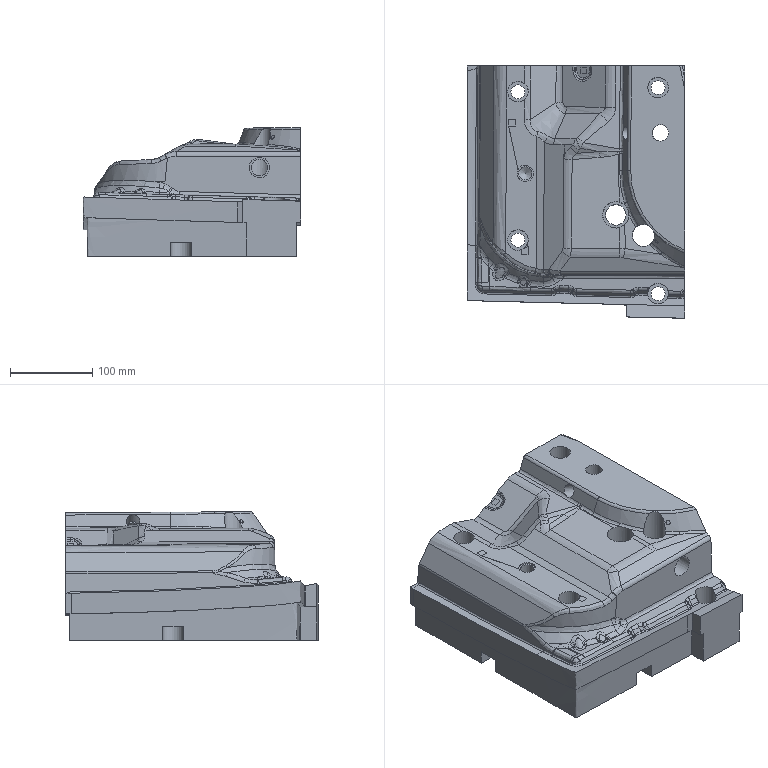Part | NX | features solid 2 | 1 solid | 279 faces | box 263.636 x 306.212 x 156.172 mm | volume 8151006 mm3 | spline 230 | plane 25 | cylinder 23 | cone 1 | commonest cylinder face diameters 25 x8 17 x4 20 x3 16 x2 35 x2 13 x1